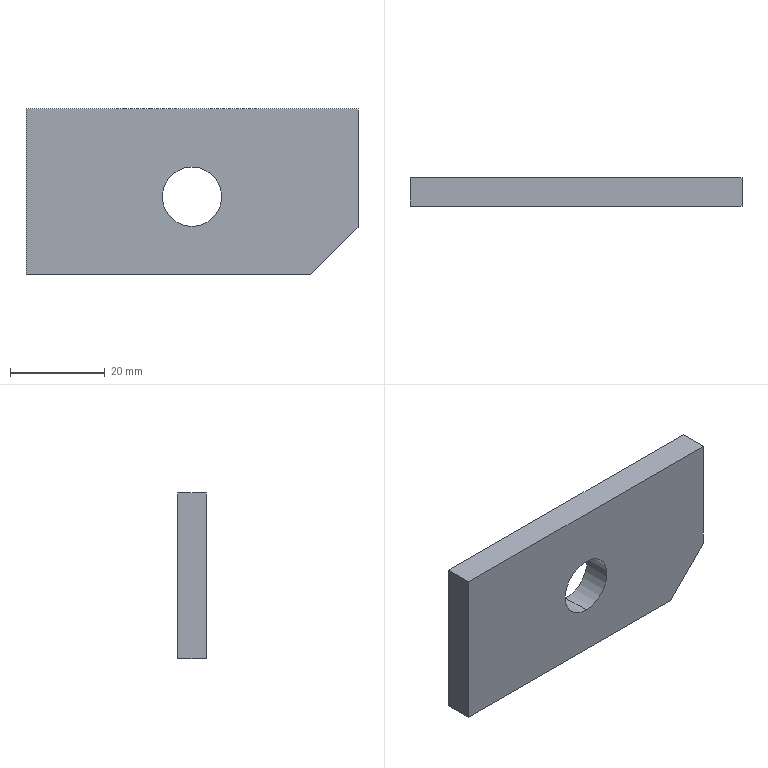Part | SolidWorks | features FlatPattern 1, SMBaseFlange 1, SheetMetal 1 | 1 solid | 9 faces | box 70 x 6 x 35 mm | volume 13664 mm3 | plane 7 | cylinder 2 | commonest cylinder face diameters 12.5 x2
STEP:
#1=CARTESIAN_POINT('',(35.,6.,-24.75));
#2=VERTEX_POINT('',#1);
#3=CARTESIAN_POINT('',(35.,6.,-12.25));
#4=VERTEX_POINT('',#3);
#5=CARTESIAN_POINT('',(35.,6.,-18.5));
#6=DIRECTION('',(0.,1.,0.));
#7=DIRECTION('',(0.,0.,1.));
#8=AXIS2_PLACEMENT_3D('',#5,#6,#7);
#9=CIRCLE('',#8,6.25);
#10=EDGE_CURVE('',#2,#4,#9,.T.);
#11=ORIENTED_EDGE('',*,*,#10,.T.);
#12=CARTESIAN_POINT('',(35.,0.,-12.25));
#13=VERTEX_POINT('',#12);
#14=CARTESIAN_POINT('',(35.,6.,-12.25));
#15=DIRECTION('',(0.,-1.,0.));
#16=VECTOR('',#15,1000.);
#17=LINE('',#14,#16);
#18=EDGE_CURVE('',#4,#13,#17,.T.);
#19=ORIENTED_EDGE('',*,*,#18,.T.);
#20=CARTESIAN_POINT('',(35.,0.,-24.75));
#21=VERTEX_POINT('',#20);
#22=CARTESIAN_POINT('',(35.,0.,-18.5));
#23=DIRECTION('',(0.,1.,0.));
#24=DIRECTION('',(0.,0.,1.));
#25=AXIS2_PLACEMENT_3D('',#22,#23,#24);
#26=CIRCLE('',#25,6.25);
#27=EDGE_CURVE('',#21,#13,#26,.T.);
#28=ORIENTED_EDGE('',*,*,#27,.F.);
#29=CARTESIAN_POINT('',(35.,6.,-24.75));
#30=DIRECTION('',(0.,-1.,0.));
#31=VECTOR('',#30,1000.);
#32=LINE('',#29,#31);
#33=EDGE_CURVE('',#2,#21,#32,.T.);
#34=ORIENTED_EDGE('',*,*,#33,.F.);
#35=EDGE_LOOP('',(#11,#19,#28,#34));
#36=FACE_OUTER_BOUND('',#35,.T.);
#37=CARTESIAN_POINT('',(35.,6.,-18.5));
#38=DIRECTION('',(0.,-1.,0.));
#39=DIRECTION('',(0.,0.,-1.));
#40=AXIS2_PLACEMENT_3D('',#37,#38,#39);
#41=CYLINDRICAL_SURFACE('',#40,6.25);
#42=ADVANCED_FACE('',(#36),#41,.F.);
#43=CARTESIAN_POINT('',(0.,6.,-35.));
#44=VERTEX_POINT('',#43);
#45=CARTESIAN_POINT('',(0.,6.,0.));
#46=VERTEX_POINT('',#45);
#47=CARTESIAN_POINT('',(0.,6.,0.));
#48=DIRECTION('',(0.,0.,1.));
#49=VECTOR('',#48,1000.);
#50=LINE('',#47,#49);
#51=EDGE_CURVE('',#44,#46,#50,.T.);
#52=ORIENTED_EDGE('',*,*,#51,.T.);
#53=CARTESIAN_POINT('',(70.,6.,0.));
#54=VERTEX_POINT('',#53);
#55=CARTESIAN_POINT('',(0.,6.,0.));
#56=DIRECTION('',(1.,0.,0.));
#57=VECTOR('',#56,1000.);
#58=LINE('',#55,#57);
#59=EDGE_CURVE('',#46,#54,#58,.T.);
#60=ORIENTED_EDGE('',*,*,#59,.T.);
#61=CARTESIAN_POINT('',(70.,6.,-25.));
#62=VERTEX_POINT('',#61);
#63=CARTESIAN_POINT('',(70.,6.,0.));
#64=DIRECTION('',(0.,0.,-1.));
#65=VECTOR('',#64,1000.);
#66=LINE('',#63,#65);
#67=EDGE_CURVE('',#54,#62,#66,.T.);
#68=ORIENTED_EDGE('',*,*,#67,.T.);
#69=CARTESIAN_POINT('',(60.,6.,-35.));
#70=VERTEX_POINT('',#69);
#71=CARTESIAN_POINT('',(60.,6.,-35.));
#72=DIRECTION('',(-0.7071,0.,-0.7071));
#73=VECTOR('',#72,1000.);
#74=LINE('',#71,#73);
#75=EDGE_CURVE('',#62,#70,#74,.T.);
#76=ORIENTED_EDGE('',*,*,#75,.T.);
#77=CARTESIAN_POINT('',(0.,6.,-35.));
#78=DIRECTION('',(-1.,0.,0.));
#79=VECTOR('',#78,1000.);
#80=LINE('',#77,#79);
#81=EDGE_CURVE('',#70,#44,#80,.T.);
#82=ORIENTED_EDGE('',*,*,#81,.T.);
#83=EDGE_LOOP('',(#52,#60,#68,#76,#82));
#84=FACE_OUTER_BOUND('',#83,.T.);
#85=ORIENTED_EDGE('',*,*,#10,.F.);
#86=CARTESIAN_POINT('',(35.,6.,-18.5));
#87=DIRECTION('',(0.,1.,0.));
#88=DIRECTION('',(0.,0.,1.));
#89=AXIS2_PLACEMENT_3D('',#86,#87,#88);
#90=CIRCLE('',#89,6.25);
#91=EDGE_CURVE('',#4,#2,#90,.T.);
#92=ORIENTED_EDGE('',*,*,#91,.F.);
#93=EDGE_LOOP('',(#85,#92));
#94=FACE_BOUND('',#93,.T.);
#95=CARTESIAN_POINT('',(0.,6.,0.));
#96=DIRECTION('',(0.,-1.,0.));
#97=DIRECTION('',(0.,0.,-1.));
#98=AXIS2_PLACEMENT_3D('',#95,#96,#97);
#99=PLANE('',#98);
#100=ADVANCED_FACE('',(#84,#94),#99,.F.);
#101=CARTESIAN_POINT('',(0.,0.,-35.));
#102=VERTEX_POINT('',#101);
#103=CARTESIAN_POINT('',(0.,0.,0.));
#104=VERTEX_POINT('',#103);
#105=CARTESIAN_POINT('',(0.,0.,0.));
#106=DIRECTION('',(0.,0.,1.));
#107=VECTOR('',#106,1000.);
#108=LINE('',#105,#107);
#109=EDGE_CURVE('',#102,#104,#108,.T.);
#110=ORIENTED_EDGE('',*,*,#109,.F.);
#111=CARTESIAN_POINT('',(60.,0.,-35.));
#112=VERTEX_POINT('',#111);
#113=CARTESIAN_POINT('',(0.,0.,-35.));
#114=DIRECTION('',(-1.,0.,0.));
#115=VECTOR('',#114,1000.);
#116=LINE('',#113,#115);
#117=EDGE_CURVE('',#112,#102,#116,.T.);
#118=ORIENTED_EDGE('',*,*,#117,.F.);
#119=CARTESIAN_POINT('',(70.,0.,-25.));
#120=VERTEX_POINT('',#119);
#121=CARTESIAN_POINT('',(60.,0.,-35.));
#122=DIRECTION('',(-0.7071,0.,-0.7071));
#123=VECTOR('',#122,1000.);
#124=LINE('',#121,#123);
#125=EDGE_CURVE('',#120,#112,#124,.T.);
#126=ORIENTED_EDGE('',*,*,#125,.F.);
#127=CARTESIAN_POINT('',(70.,0.,0.));
#128=VERTEX_POINT('',#127);
#129=CARTESIAN_POINT('',(70.,0.,0.));
#130=DIRECTION('',(0.,0.,-1.));
#131=VECTOR('',#130,1000.);
#132=LINE('',#129,#131);
#133=EDGE_CURVE('',#128,#120,#132,.T.);
#134=ORIENTED_EDGE('',*,*,#133,.F.);
#135=CARTESIAN_POINT('',(0.,0.,0.));
#136=DIRECTION('',(1.,0.,0.));
#137=VECTOR('',#136,1000.);
#138=LINE('',#135,#137);
#139=EDGE_CURVE('',#104,#128,#138,.T.);
#140=ORIENTED_EDGE('',*,*,#139,.F.);
#141=EDGE_LOOP('',(#110,#118,#126,#134,#140));
#142=FACE_OUTER_BOUND('',#141,.T.);
#143=ORIENTED_EDGE('',*,*,#27,.T.);
#144=CARTESIAN_POINT('',(35.,0.,-18.5));
#145=DIRECTION('',(0.,1.,0.));
#146=DIRECTION('',(0.,0.,1.));
#147=AXIS2_PLACEMENT_3D('',#144,#145,#146);
#148=CIRCLE('',#147,6.25);
#149=EDGE_CURVE('',#13,#21,#148,.T.);
#150=ORIENTED_EDGE('',*,*,#149,.T.);
#151=EDGE_LOOP('',(#143,#150));
#152=FACE_BOUND('',#151,.T.);
#153=CARTESIAN_POINT('',(0.,0.,0.));
#154=DIRECTION('',(0.,-1.,0.));
#155=DIRECTION('',(0.,0.,-1.));
#156=AXIS2_PLACEMENT_3D('',#153,#154,#155);
#157=PLANE('',#156);
#158=ADVANCED_FACE('',(#142,#152),#157,.T.);
#159=ORIENTED_EDGE('',*,*,#109,.T.);
#160=CARTESIAN_POINT('',(0.,6.,0.));
#161=DIRECTION('',(0.,-1.,0.));
#162=VECTOR('',#161,1000.);
#163=LINE('',#160,#162);
#164=EDGE_CURVE('',#46,#104,#163,.T.);
#165=ORIENTED_EDGE('',*,*,#164,.F.);
#166=ORIENTED_EDGE('',*,*,#51,.F.);
#167=CARTESIAN_POINT('',(0.,6.,-35.));
#168=DIRECTION('',(0.,-1.,0.));
#169=VECTOR('',#168,1000.);
#170=LINE('',#167,#169);
#171=EDGE_CURVE('',#44,#102,#170,.T.);
#172=ORIENTED_EDGE('',*,*,#171,.T.);
#173=EDGE_LOOP('',(#159,#165,#166,#172));
#174=FACE_OUTER_BOUND('',#173,.T.);
#175=CARTESIAN_POINT('',(0.,6.,0.));
#176=DIRECTION('',(1.,0.,0.));
#177=DIRECTION('',(0.,0.,-1.));
#178=AXIS2_PLACEMENT_3D('',#175,#176,#177);
#179=PLANE('',#178);
#180=ADVANCED_FACE('',(#174),#179,.F.);
#181=ORIENTED_EDGE('',*,*,#139,.T.);
#182=CARTESIAN_POINT('',(70.,6.,0.));
#183=DIRECTION('',(0.,-1.,0.));
#184=VECTOR('',#183,1000.);
#185=LINE('',#182,#184);
#186=EDGE_CURVE('',#54,#128,#185,.T.);
#187=ORIENTED_EDGE('',*,*,#186,.F.);
#188=ORIENTED_EDGE('',*,*,#59,.F.);
#189=ORIENTED_EDGE('',*,*,#164,.T.);
#190=EDGE_LOOP('',(#181,#187,#188,#189));
#191=FACE_OUTER_BOUND('',#190,.T.);
#192=CARTESIAN_POINT('',(0.,6.,0.));
#193=DIRECTION('',(0.,0.,-1.));
#194=DIRECTION('',(-1.,0.,0.));
#195=AXIS2_PLACEMENT_3D('',#192,#193,#194);
#196=PLANE('',#195);
#197=ADVANCED_FACE('',(#191),#196,.F.);
#198=ORIENTED_EDGE('',*,*,#133,.T.);
#199=CARTESIAN_POINT('',(70.,6.,-25.));
#200=DIRECTION('',(0.,-1.,0.));
#201=VECTOR('',#200,1000.);
#202=LINE('',#199,#201);
#203=EDGE_CURVE('',#62,#120,#202,.T.);
#204=ORIENTED_EDGE('',*,*,#203,.F.);
#205=ORIENTED_EDGE('',*,*,#67,.F.);
#206=ORIENTED_EDGE('',*,*,#186,.T.);
#207=EDGE_LOOP('',(#198,#204,#205,#206));
#208=FACE_OUTER_BOUND('',#207,.T.);
#209=CARTESIAN_POINT('',(70.,6.,0.));
#210=DIRECTION('',(-1.,0.,0.));
#211=DIRECTION('',(0.,0.,1.));
#212=AXIS2_PLACEMENT_3D('',#209,#210,#211);
#213=PLANE('',#212);
#214=ADVANCED_FACE('',(#208),#213,.F.);
#215=ORIENTED_EDGE('',*,*,#125,.T.);
#216=CARTESIAN_POINT('',(60.,6.,-35.));
#217=DIRECTION('',(0.,-1.,0.));
#218=VECTOR('',#217,1000.);
#219=LINE('',#216,#218);
#220=EDGE_CURVE('',#70,#112,#219,.T.);
#221=ORIENTED_EDGE('',*,*,#220,.F.);
#222=ORIENTED_EDGE('',*,*,#75,.F.);
#223=ORIENTED_EDGE('',*,*,#203,.T.);
#224=EDGE_LOOP('',(#215,#221,#222,#223));
#225=FACE_OUTER_BOUND('',#224,.T.);
#226=CARTESIAN_POINT('',(60.,6.,-35.));
#227=DIRECTION('',(-0.7071,0.,0.7071));
#228=DIRECTION('',(0.7071,0.,0.7071));
#229=AXIS2_PLACEMENT_3D('',#226,#227,#228);
#230=PLANE('',#229);
#231=ADVANCED_FACE('',(#225),#230,.F.);
#232=ORIENTED_EDGE('',*,*,#117,.T.);
#233=ORIENTED_EDGE('',*,*,#171,.F.);
#234=ORIENTED_EDGE('',*,*,#81,.F.);
#235=ORIENTED_EDGE('',*,*,#220,.T.);
#236=EDGE_LOOP('',(#232,#233,#234,#235));
#237=FACE_OUTER_BOUND('',#236,.T.);
#238=CARTESIAN_POINT('',(0.,6.,-35.));
#239=DIRECTION('',(0.,0.,1.));
#240=DIRECTION('',(1.,0.,0.));
#241=AXIS2_PLACEMENT_3D('',#238,#239,#240);
#242=PLANE('',#241);
#243=ADVANCED_FACE('',(#237),#242,.F.);
#244=ORIENTED_EDGE('',*,*,#18,.F.);
#245=ORIENTED_EDGE('',*,*,#91,.T.);
#246=ORIENTED_EDGE('',*,*,#33,.T.);
#247=ORIENTED_EDGE('',*,*,#149,.F.);
#248=EDGE_LOOP('',(#244,#245,#246,#247));
#249=FACE_OUTER_BOUND('',#248,.T.);
#250=CARTESIAN_POINT('',(35.,6.,-18.5));
#251=DIRECTION('',(0.,-1.,0.));
#252=DIRECTION('',(0.,0.,-1.));
#253=AXIS2_PLACEMENT_3D('',#250,#251,#252);
#254=CYLINDRICAL_SURFACE('',#253,6.25);
#255=ADVANCED_FACE('',(#249),#254,.F.);
#256=CLOSED_SHELL('',(#42,#100,#158,#180,#197,#214,#231,#243,#255));
#257=MANIFOLD_SOLID_BREP('',#256);
#258=CARTESIAN_POINT('',(0.,0.,0.));
#259=DIRECTION('',(0.,0.,1.));
#260=DIRECTION('',(1.,0.,0.));
#261=AXIS2_PLACEMENT_3D('',#258,#259,#260);
#262=(LENGTH_UNIT()NAMED_UNIT(*)SI_UNIT(.MILLI.,.METRE.));
#263=UNCERTAINTY_MEASURE_WITH_UNIT(LENGTH_MEASURE(0.00001),#262,'','');
#264=(NAMED_UNIT(*)PLANE_ANGLE_UNIT()SI_UNIT($,.RADIAN.));
#265=(NAMED_UNIT(*)SI_UNIT($,.STERADIAN.)SOLID_ANGLE_UNIT());
#266=(GEOMETRIC_REPRESENTATION_CONTEXT(3)GLOBAL_UNCERTAINTY_ASSIGNED_CONTEXT((#263))GLOBAL_UNIT_ASSIGNED_CONTEXT((#262,#264,#265))REPRESENTATION_CONTEXT('',''));
#267=ADVANCED_BREP_SHAPE_REPRESENTATION('',(#257,#261),#266);